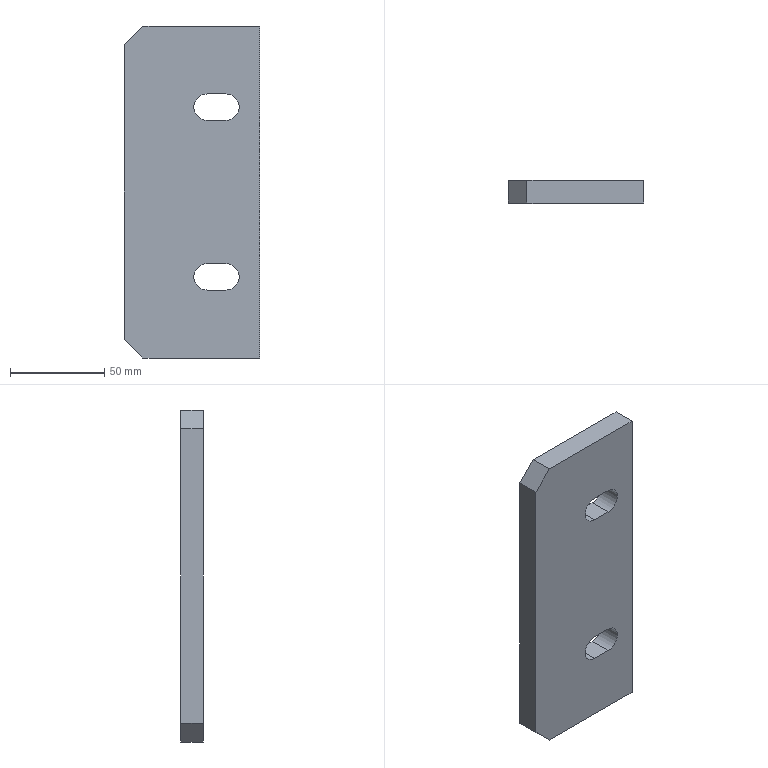Part | STEP file | 运输筋Plate 2 | 1 solid | 16 faces | box 72 x 12 x 176 mm | volume 143809 mm3 | plane 12 | cylinder 4 | commonest cylinder face diameters 14 x4
STEP:
#1=CARTESIAN_POINT('',(0.,0.,0.));
#2=DIRECTION('',(0.,0.,1.));
#3=DIRECTION('',(1.,0.,0.));
#4=AXIS2_PLACEMENT_3D('',#1,#2,#3);
#5=CARTESIAN_POINT('',(36.,0.,88.));
#6=VERTEX_POINT('',#5);
#7=CARTESIAN_POINT('',(36.,0.,-88.));
#8=VERTEX_POINT('',#7);
#9=CARTESIAN_POINT('',(36.,0.,-88.));
#10=DIRECTION('',(0.,0.,-1.));
#11=VECTOR('',#10,1.);
#12=LINE('',#9,#11);
#13=CARTESIAN_POINT('',(36.,12.,-88.));
#14=DIRECTION('',(-1.,0.,0.));
#15=DIRECTION('',(0.,0.,1.));
#16=AXIS2_PLACEMENT_3D('',#13,#14,#15);
#17=PLANE('',#16);
#18=CARTESIAN_POINT('',(0.,-12.));
#19=DIRECTION('',(-1.,0.));
#20=VECTOR('',#19,1.);
#21=LINE('',#18,#20);
#22=(GEOMETRIC_REPRESENTATION_CONTEXT(2)PARAMETRIC_REPRESENTATION_CONTEXT()REPRESENTATION_CONTEXT('',''));
#23=DEFINITIONAL_REPRESENTATION('',(#21),#22);
#24=PCURVE('',#17,#23);
#25=CARTESIAN_POINT('',(0.,0.,0.));
#26=DIRECTION('',(0.,1.,0.));
#27=DIRECTION('',(0.,0.,1.));
#28=AXIS2_PLACEMENT_3D('',#25,#26,#27);
#29=PLANE('',#28);
#30=CARTESIAN_POINT('',(-88.,36.));
#31=DIRECTION('',(-1.,0.));
#32=VECTOR('',#31,1.);
#33=LINE('',#30,#32);
#34=(GEOMETRIC_REPRESENTATION_CONTEXT(2)PARAMETRIC_REPRESENTATION_CONTEXT()REPRESENTATION_CONTEXT('',''));
#35=DEFINITIONAL_REPRESENTATION('',(#33),#34);
#36=PCURVE('',#29,#35);
#37=SURFACE_CURVE('',#12,(#24,#36),.PCURVE_S1.);
#38=EDGE_CURVE('',#6,#8,#37,.T.);
#39=ORIENTED_EDGE('',*,*,#38,.T.);
#40=CARTESIAN_POINT('',(36.,12.,-88.));
#41=VERTEX_POINT('',#40);
#42=CARTESIAN_POINT('',(36.,12.,-88.));
#43=DIRECTION('',(0.,-1.,0.));
#44=VECTOR('',#43,1.);
#45=LINE('',#42,#44);
#46=CARTESIAN_POINT('',(0.,0.));
#47=DIRECTION('',(0.,-1.));
#48=VECTOR('',#47,1.);
#49=LINE('',#46,#48);
#50=(GEOMETRIC_REPRESENTATION_CONTEXT(2)PARAMETRIC_REPRESENTATION_CONTEXT()REPRESENTATION_CONTEXT('',''));
#51=DEFINITIONAL_REPRESENTATION('',(#49),#50);
#52=PCURVE('',#17,#51);
#53=CARTESIAN_POINT('',(-36.,12.,-88.));
#54=DIRECTION('',(0.,0.,1.));
#55=DIRECTION('',(1.,0.,0.));
#56=AXIS2_PLACEMENT_3D('',#53,#54,#55);
#57=PLANE('',#56);
#58=CARTESIAN_POINT('',(72.,0.));
#59=DIRECTION('',(0.,-1.));
#60=VECTOR('',#59,1.);
#61=LINE('',#58,#60);
#62=(GEOMETRIC_REPRESENTATION_CONTEXT(2)PARAMETRIC_REPRESENTATION_CONTEXT()REPRESENTATION_CONTEXT('',''));
#63=DEFINITIONAL_REPRESENTATION('',(#61),#62);
#64=PCURVE('',#57,#63);
#65=SURFACE_CURVE('',#45,(#52,#64),.PCURVE_S1.);
#66=EDGE_CURVE('',#41,#8,#65,.T.);
#67=ORIENTED_EDGE('',*,*,#66,.F.);
#68=CARTESIAN_POINT('',(36.,12.,88.));
#69=VERTEX_POINT('',#68);
#70=CARTESIAN_POINT('',(36.,12.,-88.));
#71=DIRECTION('',(0.,0.,-1.));
#72=VECTOR('',#71,1.);
#73=LINE('',#70,#72);
#74=CARTESIAN_POINT('',(0.,0.));
#75=DIRECTION('',(-1.,0.));
#76=VECTOR('',#75,1.);
#77=LINE('',#74,#76);
#78=(GEOMETRIC_REPRESENTATION_CONTEXT(2)PARAMETRIC_REPRESENTATION_CONTEXT()REPRESENTATION_CONTEXT('',''));
#79=DEFINITIONAL_REPRESENTATION('',(#77),#78);
#80=PCURVE('',#17,#79);
#81=CARTESIAN_POINT('',(0.,12.,0.));
#82=DIRECTION('',(0.,1.,0.));
#83=DIRECTION('',(0.,0.,1.));
#84=AXIS2_PLACEMENT_3D('',#81,#82,#83);
#85=PLANE('',#84);
#86=CARTESIAN_POINT('',(-88.,36.));
#87=DIRECTION('',(-1.,0.));
#88=VECTOR('',#87,1.);
#89=LINE('',#86,#88);
#90=(GEOMETRIC_REPRESENTATION_CONTEXT(2)PARAMETRIC_REPRESENTATION_CONTEXT()REPRESENTATION_CONTEXT('',''));
#91=DEFINITIONAL_REPRESENTATION('',(#89),#90);
#92=PCURVE('',#85,#91);
#93=SURFACE_CURVE('',#73,(#80,#92),.PCURVE_S1.);
#94=EDGE_CURVE('',#69,#41,#93,.T.);
#95=ORIENTED_EDGE('',*,*,#94,.F.);
#96=CARTESIAN_POINT('',(36.,12.,88.));
#97=DIRECTION('',(0.,-1.,0.));
#98=VECTOR('',#97,1.);
#99=LINE('',#96,#98);
#100=CARTESIAN_POINT('',(176.,0.));
#101=DIRECTION('',(0.,-1.));
#102=VECTOR('',#101,1.);
#103=LINE('',#100,#102);
#104=(GEOMETRIC_REPRESENTATION_CONTEXT(2)PARAMETRIC_REPRESENTATION_CONTEXT()REPRESENTATION_CONTEXT('',''));
#105=DEFINITIONAL_REPRESENTATION('',(#103),#104);
#106=PCURVE('',#17,#105);
#107=CARTESIAN_POINT('',(-36.,12.,88.));
#108=DIRECTION('',(0.,0.,-1.));
#109=DIRECTION('',(-1.,0.,0.));
#110=AXIS2_PLACEMENT_3D('',#107,#108,#109);
#111=PLANE('',#110);
#112=CARTESIAN_POINT('',(-72.,0.));
#113=DIRECTION('',(0.,-1.));
#114=VECTOR('',#113,1.);
#115=LINE('',#112,#114);
#116=(GEOMETRIC_REPRESENTATION_CONTEXT(2)PARAMETRIC_REPRESENTATION_CONTEXT()REPRESENTATION_CONTEXT('',''));
#117=DEFINITIONAL_REPRESENTATION('',(#115),#116);
#118=PCURVE('',#111,#117);
#119=SURFACE_CURVE('',#99,(#106,#118),.PCURVE_S1.);
#120=EDGE_CURVE('',#69,#6,#119,.T.);
#121=ORIENTED_EDGE('',*,*,#120,.T.);
#122=EDGE_LOOP('',(#39,#67,#95,#121));
#123=FACE_BOUND('',#122,.T.);
#124=ADVANCED_FACE('',(#123),#17,.F.);
#125=CARTESIAN_POINT('',(-26.,0.,-88.));
#126=VERTEX_POINT('',#125);
#127=CARTESIAN_POINT('',(-36.,0.,-88.));
#128=DIRECTION('',(-1.,0.,0.));
#129=VECTOR('',#128,1.);
#130=LINE('',#127,#129);
#131=CARTESIAN_POINT('',(0.,-12.));
#132=DIRECTION('',(-1.,0.));
#133=VECTOR('',#132,1.);
#134=LINE('',#131,#133);
#135=(GEOMETRIC_REPRESENTATION_CONTEXT(2)PARAMETRIC_REPRESENTATION_CONTEXT()REPRESENTATION_CONTEXT('',''));
#136=DEFINITIONAL_REPRESENTATION('',(#134),#135);
#137=PCURVE('',#57,#136);
#138=CARTESIAN_POINT('',(-88.,-36.));
#139=DIRECTION('',(0.,-1.));
#140=VECTOR('',#139,1.);
#141=LINE('',#138,#140);
#142=(GEOMETRIC_REPRESENTATION_CONTEXT(2)PARAMETRIC_REPRESENTATION_CONTEXT()REPRESENTATION_CONTEXT('',''));
#143=DEFINITIONAL_REPRESENTATION('',(#141),#142);
#144=PCURVE('',#29,#143);
#145=SURFACE_CURVE('',#130,(#137,#144),.PCURVE_S1.);
#146=EDGE_CURVE('',#8,#126,#145,.T.);
#147=ORIENTED_EDGE('',*,*,#146,.T.);
#148=CARTESIAN_POINT('',(-26.,12.,-88.));
#149=VERTEX_POINT('',#148);
#150=CARTESIAN_POINT('',(-26.,12.,-88.));
#151=DIRECTION('',(0.,1.,0.));
#152=VECTOR('',#151,1.);
#153=LINE('',#150,#152);
#154=CARTESIAN_POINT('',(10.,0.));
#155=DIRECTION('',(0.,1.));
#156=VECTOR('',#155,1.);
#157=LINE('',#154,#156);
#158=(GEOMETRIC_REPRESENTATION_CONTEXT(2)PARAMETRIC_REPRESENTATION_CONTEXT()REPRESENTATION_CONTEXT('',''));
#159=DEFINITIONAL_REPRESENTATION('',(#157),#158);
#160=PCURVE('',#57,#159);
#161=CARTESIAN_POINT('',(-36.,12.,-78.));
#162=DIRECTION('',(0.7071,0.,0.7071));
#163=DIRECTION('',(0.,-1.,0.));
#164=AXIS2_PLACEMENT_3D('',#161,#162,#163);
#165=PLANE('',#164);
#166=CARTESIAN_POINT('',(0.,14.142));
#167=DIRECTION('',(-1.,0.));
#168=VECTOR('',#167,1.);
#169=LINE('',#166,#168);
#170=(GEOMETRIC_REPRESENTATION_CONTEXT(2)PARAMETRIC_REPRESENTATION_CONTEXT()REPRESENTATION_CONTEXT('',''));
#171=DEFINITIONAL_REPRESENTATION('',(#169),#170);
#172=PCURVE('',#165,#171);
#173=SURFACE_CURVE('',#153,(#160,#172),.PCURVE_S1.);
#174=EDGE_CURVE('',#126,#149,#173,.T.);
#175=ORIENTED_EDGE('',*,*,#174,.T.);
#176=CARTESIAN_POINT('',(-36.,12.,-88.));
#177=DIRECTION('',(-1.,0.,0.));
#178=VECTOR('',#177,1.);
#179=LINE('',#176,#178);
#180=CARTESIAN_POINT('',(0.,0.));
#181=DIRECTION('',(-1.,0.));
#182=VECTOR('',#181,1.);
#183=LINE('',#180,#182);
#184=(GEOMETRIC_REPRESENTATION_CONTEXT(2)PARAMETRIC_REPRESENTATION_CONTEXT()REPRESENTATION_CONTEXT('',''));
#185=DEFINITIONAL_REPRESENTATION('',(#183),#184);
#186=PCURVE('',#57,#185);
#187=CARTESIAN_POINT('',(-88.,-36.));
#188=DIRECTION('',(0.,-1.));
#189=VECTOR('',#188,1.);
#190=LINE('',#187,#189);
#191=(GEOMETRIC_REPRESENTATION_CONTEXT(2)PARAMETRIC_REPRESENTATION_CONTEXT()REPRESENTATION_CONTEXT('',''));
#192=DEFINITIONAL_REPRESENTATION('',(#190),#191);
#193=PCURVE('',#85,#192);
#194=SURFACE_CURVE('',#179,(#186,#193),.PCURVE_S1.);
#195=EDGE_CURVE('',#41,#149,#194,.T.);
#196=ORIENTED_EDGE('',*,*,#195,.F.);
#197=ORIENTED_EDGE('',*,*,#66,.T.);
#198=EDGE_LOOP('',(#147,#175,#196,#197));
#199=FACE_BOUND('',#198,.T.);
#200=ADVANCED_FACE('',(#199),#57,.F.);
#201=CARTESIAN_POINT('',(-36.,0.,-78.));
#202=VERTEX_POINT('',#201);
#203=CARTESIAN_POINT('',(-36.,0.,78.));
#204=VERTEX_POINT('',#203);
#205=CARTESIAN_POINT('',(-36.,0.,-88.));
#206=DIRECTION('',(0.,0.,1.));
#207=VECTOR('',#206,1.);
#208=LINE('',#205,#207);
#209=CARTESIAN_POINT('',(-36.,12.,-88.));
#210=DIRECTION('',(1.,0.,0.));
#211=DIRECTION('',(0.,0.,-1.));
#212=AXIS2_PLACEMENT_3D('',#209,#210,#211);
#213=PLANE('',#212);
#214=CARTESIAN_POINT('',(0.,-12.));
#215=DIRECTION('',(-1.,0.));
#216=VECTOR('',#215,1.);
#217=LINE('',#214,#216);
#218=(GEOMETRIC_REPRESENTATION_CONTEXT(2)PARAMETRIC_REPRESENTATION_CONTEXT()REPRESENTATION_CONTEXT('',''));
#219=DEFINITIONAL_REPRESENTATION('',(#217),#218);
#220=PCURVE('',#213,#219);
#221=CARTESIAN_POINT('',(-88.,-36.));
#222=DIRECTION('',(1.,0.));
#223=VECTOR('',#222,1.);
#224=LINE('',#221,#223);
#225=(GEOMETRIC_REPRESENTATION_CONTEXT(2)PARAMETRIC_REPRESENTATION_CONTEXT()REPRESENTATION_CONTEXT('',''));
#226=DEFINITIONAL_REPRESENTATION('',(#224),#225);
#227=PCURVE('',#29,#226);
#228=SURFACE_CURVE('',#208,(#220,#227),.PCURVE_S1.);
#229=EDGE_CURVE('',#202,#204,#228,.T.);
#230=ORIENTED_EDGE('',*,*,#229,.T.);
#231=CARTESIAN_POINT('',(-36.,12.,78.));
#232=VERTEX_POINT('',#231);
#233=CARTESIAN_POINT('',(-36.,12.,78.));
#234=DIRECTION('',(0.,1.,0.));
#235=VECTOR('',#234,1.);
#236=LINE('',#233,#235);
#237=CARTESIAN_POINT('',(-166.,0.));
#238=DIRECTION('',(0.,1.));
#239=VECTOR('',#238,1.);
#240=LINE('',#237,#239);
#241=(GEOMETRIC_REPRESENTATION_CONTEXT(2)PARAMETRIC_REPRESENTATION_CONTEXT()REPRESENTATION_CONTEXT('',''));
#242=DEFINITIONAL_REPRESENTATION('',(#240),#241);
#243=PCURVE('',#213,#242);
#244=CARTESIAN_POINT('',(-26.,12.,88.));
#245=DIRECTION('',(0.7071,0.,-0.7071));
#246=DIRECTION('',(0.,-1.,0.));
#247=AXIS2_PLACEMENT_3D('',#244,#245,#246);
#248=PLANE('',#247);
#249=CARTESIAN_POINT('',(0.,14.142));
#250=DIRECTION('',(-1.,0.));
#251=VECTOR('',#250,1.);
#252=LINE('',#249,#251);
#253=(GEOMETRIC_REPRESENTATION_CONTEXT(2)PARAMETRIC_REPRESENTATION_CONTEXT()REPRESENTATION_CONTEXT('',''));
#254=DEFINITIONAL_REPRESENTATION('',(#252),#253);
#255=PCURVE('',#248,#254);
#256=SURFACE_CURVE('',#236,(#243,#255),.PCURVE_S1.);
#257=EDGE_CURVE('',#204,#232,#256,.T.);
#258=ORIENTED_EDGE('',*,*,#257,.T.);
#259=CARTESIAN_POINT('',(-36.,12.,-78.));
#260=VERTEX_POINT('',#259);
#261=CARTESIAN_POINT('',(-36.,12.,-88.));
#262=DIRECTION('',(0.,0.,1.));
#263=VECTOR('',#262,1.);
#264=LINE('',#261,#263);
#265=CARTESIAN_POINT('',(0.,0.));
#266=DIRECTION('',(-1.,0.));
#267=VECTOR('',#266,1.);
#268=LINE('',#265,#267);
#269=(GEOMETRIC_REPRESENTATION_CONTEXT(2)PARAMETRIC_REPRESENTATION_CONTEXT()REPRESENTATION_CONTEXT('',''));
#270=DEFINITIONAL_REPRESENTATION('',(#268),#269);
#271=PCURVE('',#213,#270);
#272=CARTESIAN_POINT('',(-88.,-36.));
#273=DIRECTION('',(1.,0.));
#274=VECTOR('',#273,1.);
#275=LINE('',#272,#274);
#276=(GEOMETRIC_REPRESENTATION_CONTEXT(2)PARAMETRIC_REPRESENTATION_CONTEXT()REPRESENTATION_CONTEXT('',''));
#277=DEFINITIONAL_REPRESENTATION('',(#275),#276);
#278=PCURVE('',#85,#277);
#279=SURFACE_CURVE('',#264,(#271,#278),.PCURVE_S1.);
#280=EDGE_CURVE('',#260,#232,#279,.T.);
#281=ORIENTED_EDGE('',*,*,#280,.F.);
#282=CARTESIAN_POINT('',(-36.,12.,-78.));
#283=DIRECTION('',(0.,-1.,0.));
#284=VECTOR('',#283,1.);
#285=LINE('',#282,#284);
#286=CARTESIAN_POINT('',(-10.,0.));
#287=DIRECTION('',(0.,-1.));
#288=VECTOR('',#287,1.);
#289=LINE('',#286,#288);
#290=(GEOMETRIC_REPRESENTATION_CONTEXT(2)PARAMETRIC_REPRESENTATION_CONTEXT()REPRESENTATION_CONTEXT('',''));
#291=DEFINITIONAL_REPRESENTATION('',(#289),#290);
#292=PCURVE('',#213,#291);
#293=CARTESIAN_POINT('',(0.,0.));
#294=DIRECTION('',(1.,0.));
#295=VECTOR('',#294,1.);
#296=LINE('',#293,#295);
#297=(GEOMETRIC_REPRESENTATION_CONTEXT(2)PARAMETRIC_REPRESENTATION_CONTEXT()REPRESENTATION_CONTEXT('',''));
#298=DEFINITIONAL_REPRESENTATION('',(#296),#297);
#299=PCURVE('',#165,#298);
#300=SURFACE_CURVE('',#285,(#292,#299),.PCURVE_S1.);
#301=EDGE_CURVE('',#260,#202,#300,.T.);
#302=ORIENTED_EDGE('',*,*,#301,.T.);
#303=EDGE_LOOP('',(#230,#258,#281,#302));
#304=FACE_BOUND('',#303,.T.);
#305=ADVANCED_FACE('',(#304),#213,.F.);
#306=CARTESIAN_POINT('',(-26.,12.,88.));
#307=VERTEX_POINT('',#306);
#308=CARTESIAN_POINT('',(-36.,12.,88.));
#309=DIRECTION('',(1.,0.,0.));
#310=VECTOR('',#309,1.);
#311=LINE('',#308,#310);
#312=CARTESIAN_POINT('',(0.,0.));
#313=DIRECTION('',(-1.,0.));
#314=VECTOR('',#313,1.);
#315=LINE('',#312,#314);
#316=(GEOMETRIC_REPRESENTATION_CONTEXT(2)PARAMETRIC_REPRESENTATION_CONTEXT()REPRESENTATION_CONTEXT('',''));
#317=DEFINITIONAL_REPRESENTATION('',(#315),#316);
#318=PCURVE('',#111,#317);
#319=CARTESIAN_POINT('',(88.,-36.));
#320=DIRECTION('',(0.,1.));
#321=VECTOR('',#320,1.);
#322=LINE('',#319,#321);
#323=(GEOMETRIC_REPRESENTATION_CONTEXT(2)PARAMETRIC_REPRESENTATION_CONTEXT()REPRESENTATION_CONTEXT('',''));
#324=DEFINITIONAL_REPRESENTATION('',(#322),#323);
#325=PCURVE('',#85,#324);
#326=SURFACE_CURVE('',#311,(#318,#325),.PCURVE_S1.);
#327=EDGE_CURVE('',#307,#69,#326,.T.);
#328=ORIENTED_EDGE('',*,*,#327,.F.);
#329=CARTESIAN_POINT('',(-26.,0.,88.));
#330=VERTEX_POINT('',#329);
#331=CARTESIAN_POINT('',(-26.,12.,88.));
#332=DIRECTION('',(0.,-1.,0.));
#333=VECTOR('',#332,1.);
#334=LINE('',#331,#333);
#335=CARTESIAN_POINT('',(-10.,0.));
#336=DIRECTION('',(0.,-1.));
#337=VECTOR('',#336,1.);
#338=LINE('',#335,#337);
#339=(GEOMETRIC_REPRESENTATION_CONTEXT(2)PARAMETRIC_REPRESENTATION_CONTEXT()REPRESENTATION_CONTEXT('',''));
#340=DEFINITIONAL_REPRESENTATION('',(#338),#339);
#341=PCURVE('',#111,#340);
#342=CARTESIAN_POINT('',(0.,0.));
#343=DIRECTION('',(1.,0.));
#344=VECTOR('',#343,1.);
#345=LINE('',#342,#344);
#346=(GEOMETRIC_REPRESENTATION_CONTEXT(2)PARAMETRIC_REPRESENTATION_CONTEXT()REPRESENTATION_CONTEXT('',''));
#347=DEFINITIONAL_REPRESENTATION('',(#345),#346);
#348=PCURVE('',#248,#347);
#349=SURFACE_CURVE('',#334,(#341,#348),.PCURVE_S1.);
#350=EDGE_CURVE('',#307,#330,#349,.T.);
#351=ORIENTED_EDGE('',*,*,#350,.T.);
#352=CARTESIAN_POINT('',(-36.,0.,88.));
#353=DIRECTION('',(1.,0.,0.));
#354=VECTOR('',#353,1.);
#355=LINE('',#352,#354);
#356=CARTESIAN_POINT('',(0.,-12.));
#357=DIRECTION('',(-1.,0.));
#358=VECTOR('',#357,1.);
#359=LINE('',#356,#358);
#360=(GEOMETRIC_REPRESENTATION_CONTEXT(2)PARAMETRIC_REPRESENTATION_CONTEXT()REPRESENTATION_CONTEXT('',''));
#361=DEFINITIONAL_REPRESENTATION('',(#359),#360);
#362=PCURVE('',#111,#361);
#363=CARTESIAN_POINT('',(88.,-36.));
#364=DIRECTION('',(0.,1.));
#365=VECTOR('',#364,1.);
#366=LINE('',#363,#365);
#367=(GEOMETRIC_REPRESENTATION_CONTEXT(2)PARAMETRIC_REPRESENTATION_CONTEXT()REPRESENTATION_CONTEXT('',''));
#368=DEFINITIONAL_REPRESENTATION('',(#366),#367);
#369=PCURVE('',#29,#368);
#370=SURFACE_CURVE('',#355,(#362,#369),.PCURVE_S1.);
#371=EDGE_CURVE('',#330,#6,#370,.T.);
#372=ORIENTED_EDGE('',*,*,#371,.T.);
#373=ORIENTED_EDGE('',*,*,#120,.F.);
#374=EDGE_LOOP('',(#328,#351,#372,#373));
#375=FACE_BOUND('',#374,.T.);
#376=ADVANCED_FACE('',(#375),#111,.F.);
#377=CARTESIAN_POINT('',(8.,12.,-38.));
#378=VERTEX_POINT('',#377);
#379=CARTESIAN_POINT('',(18.,12.,-38.));
#380=VERTEX_POINT('',#379);
#381=CARTESIAN_POINT('',(8.,12.,-38.));
#382=DIRECTION('',(1.,0.,0.));
#383=VECTOR('',#382,1.);
#384=LINE('',#381,#383);
#385=CARTESIAN_POINT('',(-38.,8.));
#386=DIRECTION('',(0.,1.));
#387=VECTOR('',#386,1.);
#388=LINE('',#385,#387);
#389=(GEOMETRIC_REPRESENTATION_CONTEXT(2)PARAMETRIC_REPRESENTATION_CONTEXT()REPRESENTATION_CONTEXT('',''));
#390=DEFINITIONAL_REPRESENTATION('',(#388),#389);
#391=PCURVE('',#85,#390);
#392=CARTESIAN_POINT('',(8.,12.,-38.));
#393=DIRECTION('',(0.,0.,1.));
#394=DIRECTION('',(1.,0.,0.));
#395=AXIS2_PLACEMENT_3D('',#392,#393,#394);
#396=PLANE('',#395);
#397=CARTESIAN_POINT('',(0.,0.));
#398=DIRECTION('',(1.,0.));
#399=VECTOR('',#398,1.);
#400=LINE('',#397,#399);
#401=(GEOMETRIC_REPRESENTATION_CONTEXT(2)PARAMETRIC_REPRESENTATION_CONTEXT()REPRESENTATION_CONTEXT('',''));
#402=DEFINITIONAL_REPRESENTATION('',(#400),#401);
#403=PCURVE('',#396,#402);
#404=SURFACE_CURVE('',#384,(#391,#403),.PCURVE_S1.);
#405=EDGE_CURVE('',#378,#380,#404,.T.);
#406=ORIENTED_EDGE('',*,*,#405,.F.);
#407=CARTESIAN_POINT('',(8.,12.,-52.));
#408=VERTEX_POINT('',#407);
#409=CARTESIAN_POINT('',(8.,12.,-45.));
#410=DIRECTION('',(0.,1.,0.));
#411=DIRECTION('',(0.,0.,1.));
#412=AXIS2_PLACEMENT_3D('',#409,#410,#411);
#413=CIRCLE('',#412,7.);
#414=CARTESIAN_POINT('',(-45.,8.));
#415=DIRECTION('',(1.,0.));
#416=AXIS2_PLACEMENT_2D('',#414,#415);
#417=CIRCLE('',#416,7.);
#418=(GEOMETRIC_REPRESENTATION_CONTEXT(2)PARAMETRIC_REPRESENTATION_CONTEXT()REPRESENTATION_CONTEXT('',''));
#419=DEFINITIONAL_REPRESENTATION('',(#417),#418);
#420=PCURVE('',#85,#419);
#421=CARTESIAN_POINT('',(8.,12.,-45.));
#422=DIRECTION('',(0.,1.,0.));
#423=DIRECTION('',(0.,0.,1.));
#424=AXIS2_PLACEMENT_3D('',#421,#422,#423);
#425=CYLINDRICAL_SURFACE('',#424,7.);
#426=CARTESIAN_POINT('',(0.,0.));
#427=DIRECTION('',(1.,0.));
#428=VECTOR('',#427,1.);
#429=LINE('',#426,#428);
#430=(GEOMETRIC_REPRESENTATION_CONTEXT(2)PARAMETRIC_REPRESENTATION_CONTEXT()REPRESENTATION_CONTEXT('',''));
#431=DEFINITIONAL_REPRESENTATION('',(#429),#430);
#432=PCURVE('',#425,#431);
#433=SURFACE_CURVE('',#413,(#420,#432),.PCURVE_S1.);
#434=EDGE_CURVE('',#408,#378,#433,.T.);
#435=ORIENTED_EDGE('',*,*,#434,.F.);
#436=CARTESIAN_POINT('',(18.,12.,-52.));
#437=VERTEX_POINT('',#436);
#438=CARTESIAN_POINT('',(8.,12.,-52.));
#439=DIRECTION('',(1.,0.,0.));
#440=VECTOR('',#439,1.);
#441=LINE('',#438,#440);
#442=CARTESIAN_POINT('',(-52.,8.));
#443=DIRECTION('',(0.,1.));
#444=VECTOR('',#443,1.);
#445=LINE('',#442,#444);
#446=(GEOMETRIC_REPRESENTATION_CONTEXT(2)PARAMETRIC_REPRESENTATION_CONTEXT()REPRESENTATION_CONTEXT('',''));
#447=DEFINITIONAL_REPRESENTATION('',(#445),#446);
#448=PCURVE('',#85,#447);
#449=CARTESIAN_POINT('',(8.,12.,-52.));
#450=DIRECTION('',(0.,0.,-1.));
#451=DIRECTION('',(-1.,0.,0.));
#452=AXIS2_PLACEMENT_3D('',#449,#450,#451);
#453=PLANE('',#452);
#454=CARTESIAN_POINT('',(0.,0.));
#455=DIRECTION('',(-1.,0.));
#456=VECTOR('',#455,1.);
#457=LINE('',#454,#456);
#458=(GEOMETRIC_REPRESENTATION_CONTEXT(2)PARAMETRIC_REPRESENTATION_CONTEXT()REPRESENTATION_CONTEXT('',''));
#459=DEFINITIONAL_REPRESENTATION('',(#457),#458);
#460=PCURVE('',#453,#459);
#461=SURFACE_CURVE('',#441,(#448,#460),.PCURVE_S1.);
#462=EDGE_CURVE('',#408,#437,#461,.T.);
#463=ORIENTED_EDGE('',*,*,#462,.T.);
#464=CARTESIAN_POINT('',(18.,12.,-45.));
#465=DIRECTION('',(0.,1.,0.));
#466=DIRECTION('',(0.,0.,1.));
#467=AXIS2_PLACEMENT_3D('',#464,#465,#466);
#468=CIRCLE('',#467,7.);
#469=CARTESIAN_POINT('',(-45.,18.));
#470=DIRECTION('',(1.,0.));
#471=AXIS2_PLACEMENT_2D('',#469,#470);
#472=CIRCLE('',#471,7.);
#473=(GEOMETRIC_REPRESENTATION_CONTEXT(2)PARAMETRIC_REPRESENTATION_CONTEXT()REPRESENTATION_CONTEXT('',''));
#474=DEFINITIONAL_REPRESENTATION('',(#472),#473);
#475=PCURVE('',#85,#474);
#476=CARTESIAN_POINT('',(18.,12.,-45.));
#477=DIRECTION('',(0.,1.,0.));
#478=DIRECTION('',(0.,0.,1.));
#479=AXIS2_PLACEMENT_3D('',#476,#477,#478);
#480=CYLINDRICAL_SURFACE('',#479,7.);
#481=CARTESIAN_POINT('',(0.,0.));
#482=DIRECTION('',(1.,0.));
#483=VECTOR('',#482,1.);
#484=LINE('',#481,#483);
#485=(GEOMETRIC_REPRESENTATION_CONTEXT(2)PARAMETRIC_REPRESENTATION_CONTEXT()REPRESENTATION_CONTEXT('',''));
#486=DEFINITIONAL_REPRESENTATION('',(#484),#485);
#487=PCURVE('',#480,#486);
#488=SURFACE_CURVE('',#468,(#475,#487),.PCURVE_S1.);
#489=EDGE_CURVE('',#380,#437,#488,.T.);
#490=ORIENTED_EDGE('',*,*,#489,.F.);
#491=EDGE_LOOP('',(#406,#435,#463,#490));
#492=FACE_BOUND('',#491,.T.);
#493=CARTESIAN_POINT('',(18.,12.,52.));
#494=VERTEX_POINT('',#493);
#495=CARTESIAN_POINT('',(18.,12.,38.));
#496=VERTEX_POINT('',#495);
#497=CARTESIAN_POINT('',(18.,12.,45.));
#498=DIRECTION('',(0.,1.,0.));
#499=DIRECTION('',(0.,0.,1.));
#500=AXIS2_PLACEMENT_3D('',#497,#498,#499);
#501=CIRCLE('',#500,7.);
#502=CARTESIAN_POINT('',(45.,18.));
#503=DIRECTION('',(1.,0.));
#504=AXIS2_PLACEMENT_2D('',#502,#503);
#505=CIRCLE('',#504,7.);
#506=(GEOMETRIC_REPRESENTATION_CONTEXT(2)PARAMETRIC_REPRESENTATION_CONTEXT()REPRESENTATION_CONTEXT('',''));
#507=DEFINITIONAL_REPRESENTATION('',(#505),#506);
#508=PCURVE('',#85,#507);
#509=CARTESIAN_POINT('',(18.,12.,45.));
#510=DIRECTION('',(0.,1.,0.));
#511=DIRECTION('',(0.,0.,1.));
#512=AXIS2_PLACEMENT_3D('',#509,#510,#511);
#513=CYLINDRICAL_SURFACE('',#512,7.);
#514=CARTESIAN_POINT('',(0.,0.));
#515=DIRECTION('',(1.,0.));
#516=VECTOR('',#515,1.);
#517=LINE('',#514,#516);
#518=(GEOMETRIC_REPRESENTATION_CONTEXT(2)PARAMETRIC_REPRESENTATION_CONTEXT()REPRESENTATION_CONTEXT('',''));
#519=DEFINITIONAL_REPRESENTATION('',(#517),#518);
#520=PCURVE('',#513,#519);
#521=SURFACE_CURVE('',#501,(#508,#520),.PCURVE_S1.);
#522=EDGE_CURVE('',#494,#496,#521,.T.);
#523=ORIENTED_EDGE('',*,*,#522,.F.);
#524=CARTESIAN_POINT('',(8.,12.,52.));
#525=VERTEX_POINT('',#524);
#526=CARTESIAN_POINT('',(8.,12.,52.));
#527=DIRECTION('',(1.,0.,0.));
#528=VECTOR('',#527,1.);
#529=LINE('',#526,#528);
#530=CARTESIAN_POINT('',(52.,8.));
#531=DIRECTION('',(0.,1.));
#532=VECTOR('',#531,1.);
#533=LINE('',#530,#532);
#534=(GEOMETRIC_REPRESENTATION_CONTEXT(2)PARAMETRIC_REPRESENTATION_CONTEXT()REPRESENTATION_CONTEXT('',''));
#535=DEFINITIONAL_REPRESENTATION('',(#533),#534);
#536=PCURVE('',#85,#535);
#537=CARTESIAN_POINT('',(8.,12.,52.));
#538=DIRECTION('',(0.,0.,1.));
#539=DIRECTION('',(1.,0.,0.));
#540=AXIS2_PLACEMENT_3D('',#537,#538,#539);
#541=PLANE('',#540);
#542=CARTESIAN_POINT('',(0.,0.));
#543=DIRECTION('',(1.,0.));
#544=VECTOR('',#543,1.);
#545=LINE('',#542,#544);
#546=(GEOMETRIC_REPRESENTATION_CONTEXT(2)PARAMETRIC_REPRESENTATION_CONTEXT()REPRESENTATION_CONTEXT('',''));
#547=DEFINITIONAL_REPRESENTATION('',(#545),#546);
#548=PCURVE('',#541,#547);
#549=SURFACE_CURVE('',#529,(#536,#548),.PCURVE_S1.);
#550=EDGE_CURVE('',#525,#494,#549,.T.);
#551=ORIENTED_EDGE('',*,*,#550,.F.);
#552=CARTESIAN_POINT('',(8.,12.,38.));
#553=VERTEX_POINT('',#552);
#554=CARTESIAN_POINT('',(8.,12.,45.));
#555=DIRECTION('',(0.,1.,0.));
#556=DIRECTION('',(0.,0.,1.));
#557=AXIS2_PLACEMENT_3D('',#554,#555,#556);
#558=CIRCLE('',#557,7.);
#559=CARTESIAN_POINT('',(45.,8.));
#560=DIRECTION('',(1.,0.));
#561=AXIS2_PLACEMENT_2D('',#559,#560);
#562=CIRCLE('',#561,7.);
#563=(GEOMETRIC_REPRESENTATION_CONTEXT(2)PARAMETRIC_REPRESENTATION_CONTEXT()REPRESENTATION_CONTEXT('',''));
#564=DEFINITIONAL_REPRESENTATION('',(#562),#563);
#565=PCURVE('',#85,#564);
#566=CARTESIAN_POINT('',(8.,12.,45.));
#567=DIRECTION('',(0.,1.,0.));
#568=DIRECTION('',(0.,0.,1.));
#569=AXIS2_PLACEMENT_3D('',#566,#567,#568);
#570=CYLINDRICAL_SURFACE('',#569,7.);
#571=CARTESIAN_POINT('',(0.,0.));
#572=DIRECTION('',(1.,0.));
#573=VECTOR('',#572,1.);
#574=LINE('',#571,#573);
#575=(GEOMETRIC_REPRESENTATION_CONTEXT(2)PARAMETRIC_REPRESENTATION_CONTEXT()REPRESENTATION_CONTEXT('',''));
#576=DEFINITIONAL_REPRESENTATION('',(#574),#575);
#577=PCURVE('',#570,#576);
#578=SURFACE_CURVE('',#558,(#565,#577),.PCURVE_S1.);
#579=EDGE_CURVE('',#553,#525,#578,.T.);
#580=ORIENTED_EDGE('',*,*,#579,.F.);
#581=CARTESIAN_POINT('',(8.,12.,38.));
#582=DIRECTION('',(1.,0.,0.));
#583=VECTOR('',#582,1.);
#584=LINE('',#581,#583);
#585=CARTESIAN_POINT('',(38.,8.));
#586=DIRECTION('',(0.,1.));
#587=VECTOR('',#586,1.);
#588=LINE('',#585,#587);
#589=(GEOMETRIC_REPRESENTATION_CONTEXT(2)PARAMETRIC_REPRESENTATION_CONTEXT()REPRESENTATION_CONTEXT('',''));
#590=DEFINITIONAL_REPRESENTATION('',(#588),#589);
#591=PCURVE('',#85,#590);
#592=CARTESIAN_POINT('',(8.,12.,38.));
#593=DIRECTION('',(0.,0.,-1.));
#594=DIRECTION('',(-1.,0.,0.));
#595=AXIS2_PLACEMENT_3D('',#592,#593,#594);
#596=PLANE('',#595);
#597=CARTESIAN_POINT('',(0.,0.));
#598=DIRECTION('',(-1.,0.));
#599=VECTOR('',#598,1.);
#600=LINE('',#597,#599);
#601=(GEOMETRIC_REPRESENTATION_CONTEXT(2)PARAMETRIC_REPRESENTATION_CONTEXT()REPRESENTATION_CONTEXT('',''));
#602=DEFINITIONAL_REPRESENTATION('',(#600),#601);
#603=PCURVE('',#596,#602);
#604=SURFACE_CURVE('',#584,(#591,#603),.PCURVE_S1.);
#605=EDGE_CURVE('',#553,#496,#604,.T.);
#606=ORIENTED_EDGE('',*,*,#605,.T.);
#607=EDGE_LOOP('',(#523,#551,#580,#606));
#608=FACE_BOUND('',#607,.T.);
#609=ORIENTED_EDGE('',*,*,#280,.T.);
#610=CARTESIAN_POINT('',(-57.,12.,57.));
#611=DIRECTION('',(0.7071,0.,0.7071));
#612=VECTOR('',#611,1.);
#613=LINE('',#610,#612);
#614=CARTESIAN_POINT('',(57.,-57.));
#615=DIRECTION('',(0.7071,0.7071));
#616=VECTOR('',#615,1.);
#617=LINE('',#614,#616);
#618=(GEOMETRIC_REPRESENTATION_CONTEXT(2)PARAMETRIC_REPRESENTATION_CONTEXT()REPRESENTATION_CONTEXT('',''));
#619=DEFINITIONAL_REPRESENTATION('',(#617),#618);
#620=PCURVE('',#85,#619);
#621=CARTESIAN_POINT('',(0.,43.841));
#622=DIRECTION('',(0.,-1.));
#623=VECTOR('',#622,1.);
#624=LINE('',#621,#623);
#625=(GEOMETRIC_REPRESENTATION_CONTEXT(2)PARAMETRIC_REPRESENTATION_CONTEXT()REPRESENTATION_CONTEXT('',''));
#626=DEFINITIONAL_REPRESENTATION('',(#624),#625);
#627=PCURVE('',#248,#626);
#628=SURFACE_CURVE('',#613,(#620,#627),.PCURVE_S1.);
#629=EDGE_CURVE('',#232,#307,#628,.T.);
#630=ORIENTED_EDGE('',*,*,#629,.T.);
#631=ORIENTED_EDGE('',*,*,#327,.T.);
#632=ORIENTED_EDGE('',*,*,#94,.T.);
#633=ORIENTED_EDGE('',*,*,#195,.T.);
#634=CARTESIAN_POINT('',(-57.,12.,-57.));
#635=DIRECTION('',(-0.7071,0.,0.7071));
#636=VECTOR('',#635,1.);
#637=LINE('',#634,#636);
#638=CARTESIAN_POINT('',(-57.,-57.));
#639=DIRECTION('',(0.7071,-0.7071));
#640=VECTOR('',#639,1.);
#641=LINE('',#638,#640);
#642=(GEOMETRIC_REPRESENTATION_CONTEXT(2)PARAMETRIC_REPRESENTATION_CONTEXT()REPRESENTATION_CONTEXT('',''));
#643=DEFINITIONAL_REPRESENTATION('',(#641),#642);
#644=PCURVE('',#85,#643);
#645=CARTESIAN_POINT('',(0.,-29.698));
#646=DIRECTION('',(0.,-1.));
#647=VECTOR('',#646,1.);
#648=LINE('',#645,#647);
#649=(GEOMETRIC_REPRESENTATION_CONTEXT(2)PARAMETRIC_REPRESENTATION_CONTEXT()REPRESENTATION_CONTEXT('',''));
#650=DEFINITIONAL_REPRESENTATION('',(#648),#649);
#651=PCURVE('',#165,#650);
#652=SURFACE_CURVE('',#637,(#644,#651),.PCURVE_S1.);
#653=EDGE_CURVE('',#149,#260,#652,.T.);
#654=ORIENTED_EDGE('',*,*,#653,.T.);
#655=EDGE_LOOP('',(#609,#630,#631,#632,#633,#654));
#656=FACE_BOUND('',#655,.T.);
#657=ADVANCED_FACE('',(#492,#608,#656),#85,.T.);
#658=CARTESIAN_POINT('',(8.,0.,-52.));
#659=VERTEX_POINT('',#658);
#660=CARTESIAN_POINT('',(18.,0.,-52.));
#661=VERTEX_POINT('',#660);
#662=CARTESIAN_POINT('',(8.,0.,-52.));
#663=DIRECTION('',(1.,0.,0.));
#664=VECTOR('',#663,1.);
#665=LINE('',#662,#664);
#666=CARTESIAN_POINT('',(-52.,8.));
#667=DIRECTION('',(0.,1.));
#668=VECTOR('',#667,1.);
#669=LINE('',#666,#668);
#670=(GEOMETRIC_REPRESENTATION_CONTEXT(2)PARAMETRIC_REPRESENTATION_CONTEXT()REPRESENTATION_CONTEXT('',''));
#671=DEFINITIONAL_REPRESENTATION('',(#669),#670);
#672=PCURVE('',#29,#671);
#673=CARTESIAN_POINT('',(0.,-12.));
#674=DIRECTION('',(-1.,0.));
#675=VECTOR('',#674,1.);
#676=LINE('',#673,#675);
#677=(GEOMETRIC_REPRESENTATION_CONTEXT(2)PARAMETRIC_REPRESENTATION_CONTEXT()REPRESENTATION_CONTEXT('',''));
#678=DEFINITIONAL_REPRESENTATION('',(#676),#677);
#679=PCURVE('',#453,#678);
#680=SURFACE_CURVE('',#665,(#672,#679),.PCURVE_S1.);
#681=EDGE_CURVE('',#659,#661,#680,.T.);
#682=ORIENTED_EDGE('',*,*,#681,.F.);
#683=CARTESIAN_POINT('',(8.,0.,-38.));
#684=VERTEX_POINT('',#683);
#685=CARTESIAN_POINT('',(8.,0.,-45.));
#686=DIRECTION('',(0.,1.,0.));
#687=DIRECTION('',(0.,0.,1.));
#688=AXIS2_PLACEMENT_3D('',#685,#686,#687);
#689=CIRCLE('',#688,7.);
#690=CARTESIAN_POINT('',(-45.,8.));
#691=DIRECTION('',(1.,0.));
#692=AXIS2_PLACEMENT_2D('',#690,#691);
#693=CIRCLE('',#692,7.);
#694=(GEOMETRIC_REPRESENTATION_CONTEXT(2)PARAMETRIC_REPRESENTATION_CONTEXT()REPRESENTATION_CONTEXT('',''));
#695=DEFINITIONAL_REPRESENTATION('',(#693),#694);
#696=PCURVE('',#29,#695);
#697=CARTESIAN_POINT('',(0.,-12.));
#698=DIRECTION('',(1.,0.));
#699=VECTOR('',#698,1.);
#700=LINE('',#697,#699);
#701=(GEOMETRIC_REPRESENTATION_CONTEXT(2)PARAMETRIC_REPRESENTATION_CONTEXT()REPRESENTATION_CONTEXT('',''));
#702=DEFINITIONAL_REPRESENTATION('',(#700),#701);
#703=PCURVE('',#425,#702);
#704=SURFACE_CURVE('',#689,(#696,#703),.PCURVE_S1.);
#705=EDGE_CURVE('',#659,#684,#704,.T.);
#706=ORIENTED_EDGE('',*,*,#705,.T.);
#707=CARTESIAN_POINT('',(18.,0.,-38.));
#708=VERTEX_POINT('',#707);
#709=CARTESIAN_POINT('',(8.,0.,-38.));
#710=DIRECTION('',(1.,0.,0.));
#711=VECTOR('',#710,1.);
#712=LINE('',#709,#711);
#713=CARTESIAN_POINT('',(-38.,8.));
#714=DIRECTION('',(0.,1.));
#715=VECTOR('',#714,1.);
#716=LINE('',#713,#715);
#717=(GEOMETRIC_REPRESENTATION_CONTEXT(2)PARAMETRIC_REPRESENTATION_CONTEXT()REPRESENTATION_CONTEXT('',''));
#718=DEFINITIONAL_REPRESENTATION('',(#716),#717);
#719=PCURVE('',#29,#718);
#720=CARTESIAN_POINT('',(0.,-12.));
#721=DIRECTION('',(1.,0.));
#722=VECTOR('',#721,1.);
#723=LINE('',#720,#722);
#724=(GEOMETRIC_REPRESENTATION_CONTEXT(2)PARAMETRIC_REPRESENTATION_CONTEXT()REPRESENTATION_CONTEXT('',''));
#725=DEFINITIONAL_REPRESENTATION('',(#723),#724);
#726=PCURVE('',#396,#725);
#727=SURFACE_CURVE('',#712,(#719,#726),.PCURVE_S1.);
#728=EDGE_CURVE('',#684,#708,#727,.T.);
#729=ORIENTED_EDGE('',*,*,#728,.T.);
#730=CARTESIAN_POINT('',(18.,0.,-45.));
#731=DIRECTION('',(0.,1.,0.));
#732=DIRECTION('',(0.,0.,1.));
#733=AXIS2_PLACEMENT_3D('',#730,#731,#732);
#734=CIRCLE('',#733,7.);
#735=CARTESIAN_POINT('',(-45.,18.));
#736=DIRECTION('',(1.,0.));
#737=AXIS2_PLACEMENT_2D('',#735,#736);
#738=CIRCLE('',#737,7.);
#739=(GEOMETRIC_REPRESENTATION_CONTEXT(2)PARAMETRIC_REPRESENTATION_CONTEXT()REPRESENTATION_CONTEXT('',''));
#740=DEFINITIONAL_REPRESENTATION('',(#738),#739);
#741=PCURVE('',#29,#740);
#742=CARTESIAN_POINT('',(0.,-12.));
#743=DIRECTION('',(1.,0.));
#744=VECTOR('',#743,1.);
#745=LINE('',#742,#744);
#746=(GEOMETRIC_REPRESENTATION_CONTEXT(2)PARAMETRIC_REPRESENTATION_CONTEXT()REPRESENTATION_CONTEXT('',''));
#747=DEFINITIONAL_REPRESENTATION('',(#745),#746);
#748=PCURVE('',#480,#747);
#749=SURFACE_CURVE('',#734,(#741,#748),.PCURVE_S1.);
#750=EDGE_CURVE('',#708,#661,#749,.T.);
#751=ORIENTED_EDGE('',*,*,#750,.T.);
#752=EDGE_LOOP('',(#682,#706,#729,#751));
#753=FACE_BOUND('',#752,.T.);
#754=CARTESIAN_POINT('',(8.,0.,38.));
#755=VERTEX_POINT('',#754);
#756=CARTESIAN_POINT('',(8.,0.,52.));
#757=VERTEX_POINT('',#756);
#758=CARTESIAN_POINT('',(8.,0.,45.));
#759=DIRECTION('',(0.,1.,0.));
#760=DIRECTION('',(0.,0.,1.));
#761=AXIS2_PLACEMENT_3D('',#758,#759,#760);
#762=CIRCLE('',#761,7.);
#763=CARTESIAN_POINT('',(45.,8.));
#764=DIRECTION('',(1.,0.));
#765=AXIS2_PLACEMENT_2D('',#763,#764);
#766=CIRCLE('',#765,7.);
#767=(GEOMETRIC_REPRESENTATION_CONTEXT(2)PARAMETRIC_REPRESENTATION_CONTEXT()REPRESENTATION_CONTEXT('',''));
#768=DEFINITIONAL_REPRESENTATION('',(#766),#767);
#769=PCURVE('',#29,#768);
#770=CARTESIAN_POINT('',(0.,-12.));
#771=DIRECTION('',(1.,0.));
#772=VECTOR('',#771,1.);
#773=LINE('',#770,#772);
#774=(GEOMETRIC_REPRESENTATION_CONTEXT(2)PARAMETRIC_REPRESENTATION_CONTEXT()REPRESENTATION_CONTEXT('',''));
#775=DEFINITIONAL_REPRESENTATION('',(#773),#774);
#776=PCURVE('',#570,#775);
#777=SURFACE_CURVE('',#762,(#769,#776),.PCURVE_S1.);
#778=EDGE_CURVE('',#755,#757,#777,.T.);
#779=ORIENTED_EDGE('',*,*,#778,.T.);
#780=CARTESIAN_POINT('',(18.,0.,52.));
#781=VERTEX_POINT('',#780);
#782=CARTESIAN_POINT('',(8.,0.,52.));
#783=DIRECTION('',(1.,0.,0.));
#784=VECTOR('',#783,1.);
#785=LINE('',#782,#784);
#786=CARTESIAN_POINT('',(52.,8.));
#787=DIRECTION('',(0.,1.));
#788=VECTOR('',#787,1.);
#789=LINE('',#786,#788);
#790=(GEOMETRIC_REPRESENTATION_CONTEXT(2)PARAMETRIC_REPRESENTATION_CONTEXT()REPRESENTATION_CONTEXT('',''));
#791=DEFINITIONAL_REPRESENTATION('',(#789),#790);
#792=PCURVE('',#29,#791);
#793=CARTESIAN_POINT('',(0.,-12.));
#794=DIRECTION('',(1.,0.));
#795=VECTOR('',#794,1.);
#796=LINE('',#793,#795);
#797=(GEOMETRIC_REPRESENTATION_CONTEXT(2)PARAMETRIC_REPRESENTATION_CONTEXT()REPRESENTATION_CONTEXT('',''));
#798=DEFINITIONAL_REPRESENTATION('',(#796),#797);
#799=PCURVE('',#541,#798);
#800=SURFACE_CURVE('',#785,(#792,#799),.PCURVE_S1.);
#801=EDGE_CURVE('',#757,#781,#800,.T.);
#802=ORIENTED_EDGE('',*,*,#801,.T.);
#803=CARTESIAN_POINT('',(18.,0.,38.));
#804=VERTEX_POINT('',#803);
#805=CARTESIAN_POINT('',(18.,0.,45.));
#806=DIRECTION('',(0.,1.,0.));
#807=DIRECTION('',(0.,0.,1.));
#808=AXIS2_PLACEMENT_3D('',#805,#806,#807);
#809=CIRCLE('',#808,7.);
#810=CARTESIAN_POINT('',(45.,18.));
#811=DIRECTION('',(1.,0.));
#812=AXIS2_PLACEMENT_2D('',#810,#811);
#813=CIRCLE('',#812,7.);
#814=(GEOMETRIC_REPRESENTATION_CONTEXT(2)PARAMETRIC_REPRESENTATION_CONTEXT()REPRESENTATION_CONTEXT('',''));
#815=DEFINITIONAL_REPRESENTATION('',(#813),#814);
#816=PCURVE('',#29,#815);
#817=CARTESIAN_POINT('',(0.,-12.));
#818=DIRECTION('',(1.,0.));
#819=VECTOR('',#818,1.);
#820=LINE('',#817,#819);
#821=(GEOMETRIC_REPRESENTATION_CONTEXT(2)PARAMETRIC_REPRESENTATION_CONTEXT()REPRESENTATION_CONTEXT('',''));
#822=DEFINITIONAL_REPRESENTATION('',(#820),#821);
#823=PCURVE('',#513,#822);
#824=SURFACE_CURVE('',#809,(#816,#823),.PCURVE_S1.);
#825=EDGE_CURVE('',#781,#804,#824,.T.);
#826=ORIENTED_EDGE('',*,*,#825,.T.);
#827=CARTESIAN_POINT('',(8.,0.,38.));
#828=DIRECTION('',(1.,0.,0.));
#829=VECTOR('',#828,1.);
#830=LINE('',#827,#829);
#831=CARTESIAN_POINT('',(38.,8.));
#832=DIRECTION('',(0.,1.));
#833=VECTOR('',#832,1.);
#834=LINE('',#831,#833);
#835=(GEOMETRIC_REPRESENTATION_CONTEXT(2)PARAMETRIC_REPRESENTATION_CONTEXT()REPRESENTATION_CONTEXT('',''));
#836=DEFINITIONAL_REPRESENTATION('',(#834),#835);
#837=PCURVE('',#29,#836);
#838=CARTESIAN_POINT('',(0.,-12.));
#839=DIRECTION('',(-1.,0.));
#840=VECTOR('',#839,1.);
#841=LINE('',#838,#840);
#842=(GEOMETRIC_REPRESENTATION_CONTEXT(2)PARAMETRIC_REPRESENTATION_CONTEXT()REPRESENTATION_CONTEXT('',''));
#843=DEFINITIONAL_REPRESENTATION('',(#841),#842);
#844=PCURVE('',#596,#843);
#845=SURFACE_CURVE('',#830,(#837,#844),.PCURVE_S1.);
#846=EDGE_CURVE('',#755,#804,#845,.T.);
#847=ORIENTED_EDGE('',*,*,#846,.F.);
#848=EDGE_LOOP('',(#779,#802,#826,#847));
#849=FACE_BOUND('',#848,.T.);
#850=ORIENTED_EDGE('',*,*,#371,.F.);
#851=CARTESIAN_POINT('',(-26.,0.,88.));
#852=DIRECTION('',(-0.7071,0.,-0.7071));
#853=VECTOR('',#852,1.);
#854=LINE('',#851,#853);
#855=CARTESIAN_POINT('',(88.,-26.));
#856=DIRECTION('',(-0.7071,-0.7071));
#857=VECTOR('',#856,1.);
#858=LINE('',#855,#857);
#859=(GEOMETRIC_REPRESENTATION_CONTEXT(2)PARAMETRIC_REPRESENTATION_CONTEXT()REPRESENTATION_CONTEXT('',''));
#860=DEFINITIONAL_REPRESENTATION('',(#858),#859);
#861=PCURVE('',#29,#860);
#862=CARTESIAN_POINT('',(12.,0.));
#863=DIRECTION('',(0.,1.));
#864=VECTOR('',#863,1.);
#865=LINE('',#862,#864);
#866=(GEOMETRIC_REPRESENTATION_CONTEXT(2)PARAMETRIC_REPRESENTATION_CONTEXT()REPRESENTATION_CONTEXT('',''));
#867=DEFINITIONAL_REPRESENTATION('',(#865),#866);
#868=PCURVE('',#248,#867);
#869=SURFACE_CURVE('',#854,(#861,#868),.PCURVE_S1.);
#870=EDGE_CURVE('',#330,#204,#869,.T.);
#871=ORIENTED_EDGE('',*,*,#870,.T.);
#872=ORIENTED_EDGE('',*,*,#229,.F.);
#873=CARTESIAN_POINT('',(-36.,0.,-78.));
#874=DIRECTION('',(0.7071,0.,-0.7071));
#875=VECTOR('',#874,1.);
#876=LINE('',#873,#875);
#877=CARTESIAN_POINT('',(-78.,-36.));
#878=DIRECTION('',(-0.7071,0.7071));
#879=VECTOR('',#878,1.);
#880=LINE('',#877,#879);
#881=(GEOMETRIC_REPRESENTATION_CONTEXT(2)PARAMETRIC_REPRESENTATION_CONTEXT()REPRESENTATION_CONTEXT('',''));
#882=DEFINITIONAL_REPRESENTATION('',(#880),#881);
#883=PCURVE('',#29,#882);
#884=CARTESIAN_POINT('',(12.,0.));
#885=DIRECTION('',(0.,1.));
#886=VECTOR('',#885,1.);
#887=LINE('',#884,#886);
#888=(GEOMETRIC_REPRESENTATION_CONTEXT(2)PARAMETRIC_REPRESENTATION_CONTEXT()REPRESENTATION_CONTEXT('',''));
#889=DEFINITIONAL_REPRESENTATION('',(#887),#888);
#890=PCURVE('',#165,#889);
#891=SURFACE_CURVE('',#876,(#883,#890),.PCURVE_S1.);
#892=EDGE_CURVE('',#202,#126,#891,.T.);
#893=ORIENTED_EDGE('',*,*,#892,.T.);
#894=ORIENTED_EDGE('',*,*,#146,.F.);
#895=ORIENTED_EDGE('',*,*,#38,.F.);
#896=EDGE_LOOP('',(#850,#871,#872,#893,#894,#895));
#897=FACE_BOUND('',#896,.T.);
#898=ADVANCED_FACE('',(#753,#849,#897),#29,.F.);
#899=ORIENTED_EDGE('',*,*,#629,.F.);
#900=ORIENTED_EDGE('',*,*,#257,.F.);
#901=ORIENTED_EDGE('',*,*,#870,.F.);
#902=ORIENTED_EDGE('',*,*,#350,.F.);
#903=EDGE_LOOP('',(#899,#900,#901,#902));
#904=FACE_BOUND('',#903,.T.);
#905=ADVANCED_FACE('',(#904),#248,.F.);
#906=ORIENTED_EDGE('',*,*,#653,.F.);
#907=ORIENTED_EDGE('',*,*,#174,.F.);
#908=ORIENTED_EDGE('',*,*,#892,.F.);
#909=ORIENTED_EDGE('',*,*,#301,.F.);
#910=EDGE_LOOP('',(#906,#907,#908,#909));
#911=FACE_BOUND('',#910,.T.);
#912=ADVANCED_FACE('',(#911),#165,.F.);
#913=CARTESIAN_POINT('',(18.,12.,38.));
#914=DIRECTION('',(0.,1.,0.));
#915=VECTOR('',#914,1.);
#916=LINE('',#913,#915);
#917=CARTESIAN_POINT('',(3.142,0.));
#918=DIRECTION('',(0.,1.));
#919=VECTOR('',#918,1.);
#920=LINE('',#917,#919);
#921=(GEOMETRIC_REPRESENTATION_CONTEXT(2)PARAMETRIC_REPRESENTATION_CONTEXT()REPRESENTATION_CONTEXT('',''));
#922=DEFINITIONAL_REPRESENTATION('',(#920),#921);
#923=PCURVE('',#513,#922);
#924=CARTESIAN_POINT('',(-10.,0.));
#925=DIRECTION('',(0.,1.));
#926=VECTOR('',#925,1.);
#927=LINE('',#924,#926);
#928=(GEOMETRIC_REPRESENTATION_CONTEXT(2)PARAMETRIC_REPRESENTATION_CONTEXT()REPRESENTATION_CONTEXT('',''));
#929=DEFINITIONAL_REPRESENTATION('',(#927),#928);
#930=PCURVE('',#596,#929);
#931=SURFACE_CURVE('',#916,(#923,#930),.PCURVE_S1.);
#932=EDGE_CURVE('',#804,#496,#931,.T.);
#933=ORIENTED_EDGE('',*,*,#932,.T.);
#934=ORIENTED_EDGE('',*,*,#522,.F.);
#935=CARTESIAN_POINT('',(18.,12.,52.));
#936=DIRECTION('',(0.,-1.,0.));
#937=VECTOR('',#936,1.);
#938=LINE('',#935,#937);
#939=CARTESIAN_POINT('',(0.,0.));
#940=DIRECTION('',(0.,-1.));
#941=VECTOR('',#940,1.);
#942=LINE('',#939,#941);
#943=(GEOMETRIC_REPRESENTATION_CONTEXT(2)PARAMETRIC_REPRESENTATION_CONTEXT()REPRESENTATION_CONTEXT('',''));
#944=DEFINITIONAL_REPRESENTATION('',(#942),#943);
#945=PCURVE('',#513,#944);
#946=CARTESIAN_POINT('',(10.,0.));
#947=DIRECTION('',(0.,-1.));
#948=VECTOR('',#947,1.);
#949=LINE('',#946,#948);
#950=(GEOMETRIC_REPRESENTATION_CONTEXT(2)PARAMETRIC_REPRESENTATION_CONTEXT()REPRESENTATION_CONTEXT('',''));
#951=DEFINITIONAL_REPRESENTATION('',(#949),#950);
#952=PCURVE('',#541,#951);
#953=SURFACE_CURVE('',#938,(#945,#952),.PCURVE_S1.);
#954=EDGE_CURVE('',#494,#781,#953,.T.);
#955=ORIENTED_EDGE('',*,*,#954,.T.);
#956=ORIENTED_EDGE('',*,*,#825,.T.);
#957=EDGE_LOOP('',(#933,#934,#955,#956));
#958=FACE_BOUND('',#957,.F.);
#959=ADVANCED_FACE('',(#958),#513,.F.);
#960=CARTESIAN_POINT('',(8.,12.,38.));
#961=DIRECTION('',(0.,-1.,0.));
#962=VECTOR('',#961,1.);
#963=LINE('',#960,#962);
#964=CARTESIAN_POINT('',(3.142,0.));
#965=DIRECTION('',(0.,-1.));
#966=VECTOR('',#965,1.);
#967=LINE('',#964,#966);
#968=(GEOMETRIC_REPRESENTATION_CONTEXT(2)PARAMETRIC_REPRESENTATION_CONTEXT()REPRESENTATION_CONTEXT('',''));
#969=DEFINITIONAL_REPRESENTATION('',(#967),#968);
#970=PCURVE('',#570,#969);
#971=CARTESIAN_POINT('',(0.,0.));
#972=DIRECTION('',(0.,-1.));
#973=VECTOR('',#972,1.);
#974=LINE('',#971,#973);
#975=(GEOMETRIC_REPRESENTATION_CONTEXT(2)PARAMETRIC_REPRESENTATION_CONTEXT()REPRESENTATION_CONTEXT('',''));
#976=DEFINITIONAL_REPRESENTATION('',(#974),#975);
#977=PCURVE('',#596,#976);
#978=SURFACE_CURVE('',#963,(#970,#977),.PCURVE_S1.);
#979=EDGE_CURVE('',#553,#755,#978,.T.);
#980=ORIENTED_EDGE('',*,*,#979,.T.);
#981=ORIENTED_EDGE('',*,*,#778,.T.);
#982=CARTESIAN_POINT('',(8.,12.,52.));
#983=DIRECTION('',(0.,1.,0.));
#984=VECTOR('',#983,1.);
#985=LINE('',#982,#984);
#986=CARTESIAN_POINT('',(6.283,0.));
#987=DIRECTION('',(0.,1.));
#988=VECTOR('',#987,1.);
#989=LINE('',#986,#988);
#990=(GEOMETRIC_REPRESENTATION_CONTEXT(2)PARAMETRIC_REPRESENTATION_CONTEXT()REPRESENTATION_CONTEXT('',''));
#991=DEFINITIONAL_REPRESENTATION('',(#989),#990);
#992=PCURVE('',#570,#991);
#993=CARTESIAN_POINT('',(0.,0.));
#994=DIRECTION('',(0.,1.));
#995=VECTOR('',#994,1.);
#996=LINE('',#993,#995);
#997=(GEOMETRIC_REPRESENTATION_CONTEXT(2)PARAMETRIC_REPRESENTATION_CONTEXT()REPRESENTATION_CONTEXT('',''));
#998=DEFINITIONAL_REPRESENTATION('',(#996),#997);
#999=PCURVE('',#541,#998);
#1000=SURFACE_CURVE('',#985,(#992,#999),.PCURVE_S1.);
#1001=EDGE_CURVE('',#757,#525,#1000,.T.);
#1002=ORIENTED_EDGE('',*,*,#1001,.T.);
#1003=ORIENTED_EDGE('',*,*,#579,.F.);
#1004=EDGE_LOOP('',(#980,#981,#1002,#1003));
#1005=FACE_BOUND('',#1004,.F.);
#1006=ADVANCED_FACE('',(#1005),#570,.F.);
#1007=ORIENTED_EDGE('',*,*,#932,.T.);
#1008=ORIENTED_EDGE('',*,*,#605,.F.);
#1009=ORIENTED_EDGE('',*,*,#979,.T.);
#1010=ORIENTED_EDGE('',*,*,#846,.T.);
#1011=EDGE_LOOP('',(#1007,#1008,#1009,#1010));
#1012=FACE_BOUND('',#1011,.T.);
#1013=ADVANCED_FACE('',(#1012),#596,.F.);
#1014=ORIENTED_EDGE('',*,*,#954,.T.);
#1015=ORIENTED_EDGE('',*,*,#801,.F.);
#1016=ORIENTED_EDGE('',*,*,#1001,.T.);
#1017=ORIENTED_EDGE('',*,*,#550,.T.);
#1018=EDGE_LOOP('',(#1014,#1015,#1016,#1017));
#1019=FACE_BOUND('',#1018,.T.);
#1020=ADVANCED_FACE('',(#1019),#541,.F.);
#1021=CARTESIAN_POINT('',(18.,12.,-52.));
#1022=DIRECTION('',(0.,1.,0.));
#1023=VECTOR('',#1022,1.);
#1024=LINE('',#1021,#1023);
#1025=CARTESIAN_POINT('',(3.142,0.));
#1026=DIRECTION('',(0.,1.));
#1027=VECTOR('',#1026,1.);
#1028=LINE('',#1025,#1027);
#1029=(GEOMETRIC_REPRESENTATION_CONTEXT(2)PARAMETRIC_REPRESENTATION_CONTEXT()REPRESENTATION_CONTEXT('',''));
#1030=DEFINITIONAL_REPRESENTATION('',(#1028),#1029);
#1031=PCURVE('',#480,#1030);
#1032=CARTESIAN_POINT('',(-10.,0.));
#1033=DIRECTION('',(0.,1.));
#1034=VECTOR('',#1033,1.);
#1035=LINE('',#1032,#1034);
#1036=(GEOMETRIC_REPRESENTATION_CONTEXT(2)PARAMETRIC_REPRESENTATION_CONTEXT()REPRESENTATION_CONTEXT('',''));
#1037=DEFINITIONAL_REPRESENTATION('',(#1035),#1036);
#1038=PCURVE('',#453,#1037);
#1039=SURFACE_CURVE('',#1024,(#1031,#1038),.PCURVE_S1.);
#1040=EDGE_CURVE('',#661,#437,#1039,.T.);
#1041=ORIENTED_EDGE('',*,*,#1040,.T.);
#1042=ORIENTED_EDGE('',*,*,#489,.F.);
#1043=CARTESIAN_POINT('',(18.,12.,-38.));
#1044=DIRECTION('',(0.,-1.,0.));
#1045=VECTOR('',#1044,1.);
#1046=LINE('',#1043,#1045);
#1047=CARTESIAN_POINT('',(0.,0.));
#1048=DIRECTION('',(0.,-1.));
#1049=VECTOR('',#1048,1.);
#1050=LINE('',#1047,#1049);
#1051=(GEOMETRIC_REPRESENTATION_CONTEXT(2)PARAMETRIC_REPRESENTATION_CONTEXT()REPRESENTATION_CONTEXT('',''));
#1052=DEFINITIONAL_REPRESENTATION('',(#1050),#1051);
#1053=PCURVE('',#480,#1052);
#1054=CARTESIAN_POINT('',(10.,0.));
#1055=DIRECTION('',(0.,-1.));
#1056=VECTOR('',#1055,1.);
#1057=LINE('',#1054,#1056);
#1058=(GEOMETRIC_REPRESENTATION_CONTEXT(2)PARAMETRIC_REPRESENTATION_CONTEXT()REPRESENTATION_CONTEXT('',''));
#1059=DEFINITIONAL_REPRESENTATION('',(#1057),#1058);
#1060=PCURVE('',#396,#1059);
#1061=SURFACE_CURVE('',#1046,(#1053,#1060),.PCURVE_S1.);
#1062=EDGE_CURVE('',#380,#708,#1061,.T.);
#1063=ORIENTED_EDGE('',*,*,#1062,.T.);
#1064=ORIENTED_EDGE('',*,*,#750,.T.);
#1065=EDGE_LOOP('',(#1041,#1042,#1063,#1064));
#1066=FACE_BOUND('',#1065,.F.);
#1067=ADVANCED_FACE('',(#1066),#480,.F.);
#1068=CARTESIAN_POINT('',(8.,12.,-52.));
#1069=DIRECTION('',(0.,-1.,0.));
#1070=VECTOR('',#1069,1.);
#1071=LINE('',#1068,#1070);
#1072=CARTESIAN_POINT('',(3.142,0.));
#1073=DIRECTION('',(0.,-1.));
#1074=VECTOR('',#1073,1.);
#1075=LINE('',#1072,#1074);
#1076=(GEOMETRIC_REPRESENTATION_CONTEXT(2)PARAMETRIC_REPRESENTATION_CONTEXT()REPRESENTATION_CONTEXT('',''));
#1077=DEFINITIONAL_REPRESENTATION('',(#1075),#1076);
#1078=PCURVE('',#425,#1077);
#1079=CARTESIAN_POINT('',(0.,0.));
#1080=DIRECTION('',(0.,-1.));
#1081=VECTOR('',#1080,1.);
#1082=LINE('',#1079,#1081);
#1083=(GEOMETRIC_REPRESENTATION_CONTEXT(2)PARAMETRIC_REPRESENTATION_CONTEXT()REPRESENTATION_CONTEXT('',''));
#1084=DEFINITIONAL_REPRESENTATION('',(#1082),#1083);
#1085=PCURVE('',#453,#1084);
#1086=SURFACE_CURVE('',#1071,(#1078,#1085),.PCURVE_S1.);
#1087=EDGE_CURVE('',#408,#659,#1086,.T.);
#1088=ORIENTED_EDGE('',*,*,#1087,.T.);
#1089=ORIENTED_EDGE('',*,*,#705,.T.);
#1090=CARTESIAN_POINT('',(8.,12.,-38.));
#1091=DIRECTION('',(0.,1.,0.));
#1092=VECTOR('',#1091,1.);
#1093=LINE('',#1090,#1092);
#1094=CARTESIAN_POINT('',(6.283,0.));
#1095=DIRECTION('',(0.,1.));
#1096=VECTOR('',#1095,1.);
#1097=LINE('',#1094,#1096);
#1098=(GEOMETRIC_REPRESENTATION_CONTEXT(2)PARAMETRIC_REPRESENTATION_CONTEXT()REPRESENTATION_CONTEXT('',''));
#1099=DEFINITIONAL_REPRESENTATION('',(#1097),#1098);
#1100=PCURVE('',#425,#1099);
#1101=CARTESIAN_POINT('',(0.,0.));
#1102=DIRECTION('',(0.,1.));
#1103=VECTOR('',#1102,1.);
#1104=LINE('',#1101,#1103);
#1105=(GEOMETRIC_REPRESENTATION_CONTEXT(2)PARAMETRIC_REPRESENTATION_CONTEXT()REPRESENTATION_CONTEXT('',''));
#1106=DEFINITIONAL_REPRESENTATION('',(#1104),#1105);
#1107=PCURVE('',#396,#1106);
#1108=SURFACE_CURVE('',#1093,(#1100,#1107),.PCURVE_S1.);
#1109=EDGE_CURVE('',#684,#378,#1108,.T.);
#1110=ORIENTED_EDGE('',*,*,#1109,.T.);
#1111=ORIENTED_EDGE('',*,*,#434,.F.);
#1112=EDGE_LOOP('',(#1088,#1089,#1110,#1111));
#1113=FACE_BOUND('',#1112,.F.);
#1114=ADVANCED_FACE('',(#1113),#425,.F.);
#1115=ORIENTED_EDGE('',*,*,#1040,.T.);
#1116=ORIENTED_EDGE('',*,*,#462,.F.);
#1117=ORIENTED_EDGE('',*,*,#1087,.T.);
#1118=ORIENTED_EDGE('',*,*,#681,.T.);
#1119=EDGE_LOOP('',(#1115,#1116,#1117,#1118));
#1120=FACE_BOUND('',#1119,.T.);
#1121=ADVANCED_FACE('',(#1120),#453,.F.);
#1122=ORIENTED_EDGE('',*,*,#1062,.T.);
#1123=ORIENTED_EDGE('',*,*,#728,.F.);
#1124=ORIENTED_EDGE('',*,*,#1109,.T.);
#1125=ORIENTED_EDGE('',*,*,#405,.T.);
#1126=EDGE_LOOP('',(#1122,#1123,#1124,#1125));
#1127=FACE_BOUND('',#1126,.T.);
#1128=ADVANCED_FACE('',(#1127),#396,.F.);
#1129=CLOSED_SHELL('',(#124,#200,#305,#376,#657,#898,#905,#912,#959,#1006,#1013,#1020,#1067,#1114,#1121,#1128));
#1130=MANIFOLD_SOLID_BREP('',#1129);
#1131=(LENGTH_UNIT()NAMED_UNIT(*)SI_UNIT(.MILLI.,.METRE.));
#1132=UNCERTAINTY_MEASURE_WITH_UNIT(LENGTH_MEASURE(0.0000001),#1131,'','');
#1133=(NAMED_UNIT(*)PLANE_ANGLE_UNIT()SI_UNIT($,.RADIAN.));
#1134=(NAMED_UNIT(*)SI_UNIT($,.STERADIAN.)SOLID_ANGLE_UNIT());
#1135=(GEOMETRIC_REPRESENTATION_CONTEXT(3)GLOBAL_UNCERTAINTY_ASSIGNED_CONTEXT((#1132))GLOBAL_UNIT_ASSIGNED_CONTEXT((#1131,#1133,#1134))REPRESENTATION_CONTEXT('',''));
#1136=ADVANCED_BREP_SHAPE_REPRESENTATION('',(#4,#1130),#1135);